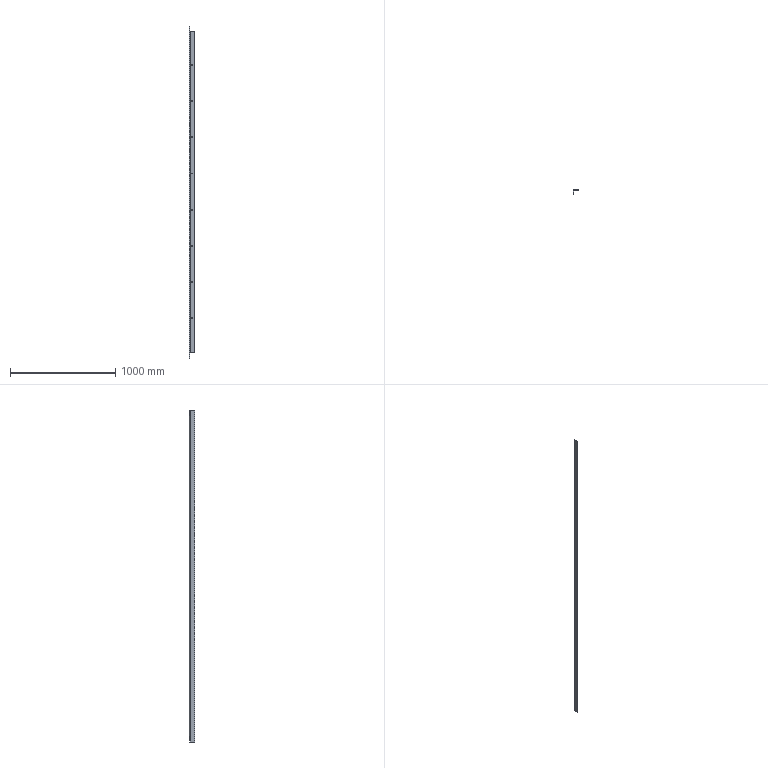Part | SolidWorks | features BaseBody 1 | 1 solid | 30 faces | box 50 x 50 x 3151 mm | volume 1714556 mm3 | cylinder 18 | plane 12 | commonest cylinder face diameters 9 x16 1.473 x1 13.473 x1
STEP:
#1=CARTESIAN_POINT('',(26.,50.,383.5));
#2=VERTEX_POINT('',#1);
#3=CARTESIAN_POINT('',(26.,50.,374.5));
#4=VERTEX_POINT('',#3);
#5=CARTESIAN_POINT('',(26.,50.,379.));
#6=DIRECTION('',(0.,-1.,0.));
#7=DIRECTION('',(0.,0.,-1.));
#8=AXIS2_PLACEMENT_3D('',#5,#6,#7);
#9=CIRCLE('',#8,4.5);
#10=EDGE_CURVE('',#2,#4,#9,.T.);
#11=ORIENTED_EDGE('',*,*,#10,.F.);
#12=CARTESIAN_POINT('',(26.,44.,383.5));
#13=VERTEX_POINT('',#12);
#14=CARTESIAN_POINT('',(26.,50.,383.5));
#15=DIRECTION('',(0.,-1.,0.));
#16=VECTOR('',#15,1000.);
#17=LINE('',#14,#16);
#18=EDGE_CURVE('',#2,#13,#17,.T.);
#19=ORIENTED_EDGE('',*,*,#18,.T.);
#20=CARTESIAN_POINT('',(26.,44.,374.5));
#21=VERTEX_POINT('',#20);
#22=CARTESIAN_POINT('',(26.,44.,379.));
#23=DIRECTION('',(0.,-1.,0.));
#24=DIRECTION('',(0.,0.,-1.));
#25=AXIS2_PLACEMENT_3D('',#22,#23,#24);
#26=CIRCLE('',#25,4.5);
#27=EDGE_CURVE('',#13,#21,#26,.T.);
#28=ORIENTED_EDGE('',*,*,#27,.T.);
#29=CARTESIAN_POINT('',(26.,50.,374.5));
#30=DIRECTION('',(0.,-1.,0.));
#31=VECTOR('',#30,1000.);
#32=LINE('',#29,#31);
#33=EDGE_CURVE('',#4,#21,#32,.T.);
#34=ORIENTED_EDGE('',*,*,#33,.F.);
#35=EDGE_LOOP('',(#11,#19,#28,#34));
#36=FACE_OUTER_BOUND('',#35,.T.);
#37=CARTESIAN_POINT('',(26.,50.,379.));
#38=DIRECTION('',(0.,-1.,0.));
#39=DIRECTION('',(0.,0.,-1.));
#40=AXIS2_PLACEMENT_3D('',#37,#38,#39);
#41=CYLINDRICAL_SURFACE('',#40,4.5);
#42=ADVANCED_FACE('',(#36),#41,.F.);
#43=CARTESIAN_POINT('',(26.,50.,726.5));
#44=VERTEX_POINT('',#43);
#45=CARTESIAN_POINT('',(26.,50.,717.5));
#46=VERTEX_POINT('',#45);
#47=CARTESIAN_POINT('',(26.,50.,722.));
#48=DIRECTION('',(0.,-1.,0.));
#49=DIRECTION('',(0.,0.,-1.));
#50=AXIS2_PLACEMENT_3D('',#47,#48,#49);
#51=CIRCLE('',#50,4.5);
#52=EDGE_CURVE('',#44,#46,#51,.T.);
#53=ORIENTED_EDGE('',*,*,#52,.F.);
#54=CARTESIAN_POINT('',(26.,44.,726.5));
#55=VERTEX_POINT('',#54);
#56=CARTESIAN_POINT('',(26.,50.,726.5));
#57=DIRECTION('',(0.,-1.,0.));
#58=VECTOR('',#57,1000.);
#59=LINE('',#56,#58);
#60=EDGE_CURVE('',#44,#55,#59,.T.);
#61=ORIENTED_EDGE('',*,*,#60,.T.);
#62=CARTESIAN_POINT('',(26.,44.,717.5));
#63=VERTEX_POINT('',#62);
#64=CARTESIAN_POINT('',(26.,44.,722.));
#65=DIRECTION('',(0.,-1.,0.));
#66=DIRECTION('',(0.,0.,-1.));
#67=AXIS2_PLACEMENT_3D('',#64,#65,#66);
#68=CIRCLE('',#67,4.5);
#69=EDGE_CURVE('',#55,#63,#68,.T.);
#70=ORIENTED_EDGE('',*,*,#69,.T.);
#71=CARTESIAN_POINT('',(26.,50.,717.5));
#72=DIRECTION('',(0.,-1.,0.));
#73=VECTOR('',#72,1000.);
#74=LINE('',#71,#73);
#75=EDGE_CURVE('',#46,#63,#74,.T.);
#76=ORIENTED_EDGE('',*,*,#75,.F.);
#77=EDGE_LOOP('',(#53,#61,#70,#76));
#78=FACE_OUTER_BOUND('',#77,.T.);
#79=CARTESIAN_POINT('',(26.,50.,722.));
#80=DIRECTION('',(0.,-1.,0.));
#81=DIRECTION('',(0.,0.,-1.));
#82=AXIS2_PLACEMENT_3D('',#79,#80,#81);
#83=CYLINDRICAL_SURFACE('',#82,4.5);
#84=ADVANCED_FACE('',(#78),#83,.F.);
#85=CARTESIAN_POINT('',(26.,50.,1069.5));
#86=VERTEX_POINT('',#85);
#87=CARTESIAN_POINT('',(26.,50.,1060.5));
#88=VERTEX_POINT('',#87);
#89=CARTESIAN_POINT('',(26.,50.,1065.));
#90=DIRECTION('',(0.,-1.,0.));
#91=DIRECTION('',(0.,0.,-1.));
#92=AXIS2_PLACEMENT_3D('',#89,#90,#91);
#93=CIRCLE('',#92,4.5);
#94=EDGE_CURVE('',#86,#88,#93,.T.);
#95=ORIENTED_EDGE('',*,*,#94,.F.);
#96=CARTESIAN_POINT('',(26.,44.,1069.5));
#97=VERTEX_POINT('',#96);
#98=CARTESIAN_POINT('',(26.,50.,1069.5));
#99=DIRECTION('',(0.,-1.,0.));
#100=VECTOR('',#99,1000.);
#101=LINE('',#98,#100);
#102=EDGE_CURVE('',#86,#97,#101,.T.);
#103=ORIENTED_EDGE('',*,*,#102,.T.);
#104=CARTESIAN_POINT('',(26.,44.,1060.5));
#105=VERTEX_POINT('',#104);
#106=CARTESIAN_POINT('',(26.,44.,1065.));
#107=DIRECTION('',(0.,-1.,0.));
#108=DIRECTION('',(0.,0.,-1.));
#109=AXIS2_PLACEMENT_3D('',#106,#107,#108);
#110=CIRCLE('',#109,4.5);
#111=EDGE_CURVE('',#97,#105,#110,.T.);
#112=ORIENTED_EDGE('',*,*,#111,.T.);
#113=CARTESIAN_POINT('',(26.,50.,1060.5));
#114=DIRECTION('',(0.,-1.,0.));
#115=VECTOR('',#114,1000.);
#116=LINE('',#113,#115);
#117=EDGE_CURVE('',#88,#105,#116,.T.);
#118=ORIENTED_EDGE('',*,*,#117,.F.);
#119=EDGE_LOOP('',(#95,#103,#112,#118));
#120=FACE_OUTER_BOUND('',#119,.T.);
#121=CARTESIAN_POINT('',(26.,50.,1065.));
#122=DIRECTION('',(0.,-1.,0.));
#123=DIRECTION('',(0.,0.,-1.));
#124=AXIS2_PLACEMENT_3D('',#121,#122,#123);
#125=CYLINDRICAL_SURFACE('',#124,4.5);
#126=ADVANCED_FACE('',(#120),#125,.F.);
#127=CARTESIAN_POINT('',(26.,50.,1412.5));
#128=VERTEX_POINT('',#127);
#129=CARTESIAN_POINT('',(26.,50.,1403.5));
#130=VERTEX_POINT('',#129);
#131=CARTESIAN_POINT('',(26.,50.,1408.));
#132=DIRECTION('',(0.,-1.,0.));
#133=DIRECTION('',(0.,0.,-1.));
#134=AXIS2_PLACEMENT_3D('',#131,#132,#133);
#135=CIRCLE('',#134,4.5);
#136=EDGE_CURVE('',#128,#130,#135,.T.);
#137=ORIENTED_EDGE('',*,*,#136,.F.);
#138=CARTESIAN_POINT('',(26.,44.,1412.5));
#139=VERTEX_POINT('',#138);
#140=CARTESIAN_POINT('',(26.,50.,1412.5));
#141=DIRECTION('',(0.,-1.,0.));
#142=VECTOR('',#141,1000.);
#143=LINE('',#140,#142);
#144=EDGE_CURVE('',#128,#139,#143,.T.);
#145=ORIENTED_EDGE('',*,*,#144,.T.);
#146=CARTESIAN_POINT('',(26.,44.,1403.5));
#147=VERTEX_POINT('',#146);
#148=CARTESIAN_POINT('',(26.,44.,1408.));
#149=DIRECTION('',(0.,-1.,0.));
#150=DIRECTION('',(0.,0.,-1.));
#151=AXIS2_PLACEMENT_3D('',#148,#149,#150);
#152=CIRCLE('',#151,4.5);
#153=EDGE_CURVE('',#139,#147,#152,.T.);
#154=ORIENTED_EDGE('',*,*,#153,.T.);
#155=CARTESIAN_POINT('',(26.,50.,1403.5));
#156=DIRECTION('',(0.,-1.,0.));
#157=VECTOR('',#156,1000.);
#158=LINE('',#155,#157);
#159=EDGE_CURVE('',#130,#147,#158,.T.);
#160=ORIENTED_EDGE('',*,*,#159,.F.);
#161=EDGE_LOOP('',(#137,#145,#154,#160));
#162=FACE_OUTER_BOUND('',#161,.T.);
#163=CARTESIAN_POINT('',(26.,50.,1408.));
#164=DIRECTION('',(0.,-1.,0.));
#165=DIRECTION('',(0.,0.,-1.));
#166=AXIS2_PLACEMENT_3D('',#163,#164,#165);
#167=CYLINDRICAL_SURFACE('',#166,4.5);
#168=ADVANCED_FACE('',(#162),#167,.F.);
#169=CARTESIAN_POINT('',(26.,50.,1755.5));
#170=VERTEX_POINT('',#169);
#171=CARTESIAN_POINT('',(26.,50.,1746.5));
#172=VERTEX_POINT('',#171);
#173=CARTESIAN_POINT('',(26.,50.,1751.));
#174=DIRECTION('',(0.,-1.,0.));
#175=DIRECTION('',(0.,0.,-1.));
#176=AXIS2_PLACEMENT_3D('',#173,#174,#175);
#177=CIRCLE('',#176,4.5);
#178=EDGE_CURVE('',#170,#172,#177,.T.);
#179=ORIENTED_EDGE('',*,*,#178,.F.);
#180=CARTESIAN_POINT('',(26.,44.,1755.5));
#181=VERTEX_POINT('',#180);
#182=CARTESIAN_POINT('',(26.,50.,1755.5));
#183=DIRECTION('',(0.,-1.,0.));
#184=VECTOR('',#183,1000.);
#185=LINE('',#182,#184);
#186=EDGE_CURVE('',#170,#181,#185,.T.);
#187=ORIENTED_EDGE('',*,*,#186,.T.);
#188=CARTESIAN_POINT('',(26.,44.,1746.5));
#189=VERTEX_POINT('',#188);
#190=CARTESIAN_POINT('',(26.,44.,1751.));
#191=DIRECTION('',(0.,-1.,0.));
#192=DIRECTION('',(0.,0.,-1.));
#193=AXIS2_PLACEMENT_3D('',#190,#191,#192);
#194=CIRCLE('',#193,4.5);
#195=EDGE_CURVE('',#181,#189,#194,.T.);
#196=ORIENTED_EDGE('',*,*,#195,.T.);
#197=CARTESIAN_POINT('',(26.,50.,1746.5));
#198=DIRECTION('',(0.,-1.,0.));
#199=VECTOR('',#198,1000.);
#200=LINE('',#197,#199);
#201=EDGE_CURVE('',#172,#189,#200,.T.);
#202=ORIENTED_EDGE('',*,*,#201,.F.);
#203=EDGE_LOOP('',(#179,#187,#196,#202));
#204=FACE_OUTER_BOUND('',#203,.T.);
#205=CARTESIAN_POINT('',(26.,50.,1751.));
#206=DIRECTION('',(0.,-1.,0.));
#207=DIRECTION('',(0.,0.,-1.));
#208=AXIS2_PLACEMENT_3D('',#205,#206,#207);
#209=CYLINDRICAL_SURFACE('',#208,4.5);
#210=ADVANCED_FACE('',(#204),#209,.F.);
#211=CARTESIAN_POINT('',(26.,50.,2098.5));
#212=VERTEX_POINT('',#211);
#213=CARTESIAN_POINT('',(26.,50.,2089.5));
#214=VERTEX_POINT('',#213);
#215=CARTESIAN_POINT('',(26.,50.,2094.));
#216=DIRECTION('',(0.,-1.,0.));
#217=DIRECTION('',(0.,0.,-1.));
#218=AXIS2_PLACEMENT_3D('',#215,#216,#217);
#219=CIRCLE('',#218,4.5);
#220=EDGE_CURVE('',#212,#214,#219,.T.);
#221=ORIENTED_EDGE('',*,*,#220,.F.);
#222=CARTESIAN_POINT('',(26.,44.,2098.5));
#223=VERTEX_POINT('',#222);
#224=CARTESIAN_POINT('',(26.,50.,2098.5));
#225=DIRECTION('',(0.,-1.,0.));
#226=VECTOR('',#225,1000.);
#227=LINE('',#224,#226);
#228=EDGE_CURVE('',#212,#223,#227,.T.);
#229=ORIENTED_EDGE('',*,*,#228,.T.);
#230=CARTESIAN_POINT('',(26.,44.,2089.5));
#231=VERTEX_POINT('',#230);
#232=CARTESIAN_POINT('',(26.,44.,2094.));
#233=DIRECTION('',(0.,-1.,0.));
#234=DIRECTION('',(0.,0.,-1.));
#235=AXIS2_PLACEMENT_3D('',#232,#233,#234);
#236=CIRCLE('',#235,4.5);
#237=EDGE_CURVE('',#223,#231,#236,.T.);
#238=ORIENTED_EDGE('',*,*,#237,.T.);
#239=CARTESIAN_POINT('',(26.,50.,2089.5));
#240=DIRECTION('',(0.,-1.,0.));
#241=VECTOR('',#240,1000.);
#242=LINE('',#239,#241);
#243=EDGE_CURVE('',#214,#231,#242,.T.);
#244=ORIENTED_EDGE('',*,*,#243,.F.);
#245=EDGE_LOOP('',(#221,#229,#238,#244));
#246=FACE_OUTER_BOUND('',#245,.T.);
#247=CARTESIAN_POINT('',(26.,50.,2094.));
#248=DIRECTION('',(0.,-1.,0.));
#249=DIRECTION('',(0.,0.,-1.));
#250=AXIS2_PLACEMENT_3D('',#247,#248,#249);
#251=CYLINDRICAL_SURFACE('',#250,4.5);
#252=ADVANCED_FACE('',(#246),#251,.F.);
#253=CARTESIAN_POINT('',(26.,50.,2441.5));
#254=VERTEX_POINT('',#253);
#255=CARTESIAN_POINT('',(26.,50.,2432.5));
#256=VERTEX_POINT('',#255);
#257=CARTESIAN_POINT('',(26.,50.,2437.));
#258=DIRECTION('',(0.,-1.,0.));
#259=DIRECTION('',(0.,0.,-1.));
#260=AXIS2_PLACEMENT_3D('',#257,#258,#259);
#261=CIRCLE('',#260,4.5);
#262=EDGE_CURVE('',#254,#256,#261,.T.);
#263=ORIENTED_EDGE('',*,*,#262,.F.);
#264=CARTESIAN_POINT('',(26.,44.,2441.5));
#265=VERTEX_POINT('',#264);
#266=CARTESIAN_POINT('',(26.,50.,2441.5));
#267=DIRECTION('',(0.,-1.,0.));
#268=VECTOR('',#267,1000.);
#269=LINE('',#266,#268);
#270=EDGE_CURVE('',#254,#265,#269,.T.);
#271=ORIENTED_EDGE('',*,*,#270,.T.);
#272=CARTESIAN_POINT('',(26.,44.,2432.5));
#273=VERTEX_POINT('',#272);
#274=CARTESIAN_POINT('',(26.,44.,2437.));
#275=DIRECTION('',(0.,-1.,0.));
#276=DIRECTION('',(0.,0.,-1.));
#277=AXIS2_PLACEMENT_3D('',#274,#275,#276);
#278=CIRCLE('',#277,4.5);
#279=EDGE_CURVE('',#265,#273,#278,.T.);
#280=ORIENTED_EDGE('',*,*,#279,.T.);
#281=CARTESIAN_POINT('',(26.,50.,2432.5));
#282=DIRECTION('',(0.,-1.,0.));
#283=VECTOR('',#282,1000.);
#284=LINE('',#281,#283);
#285=EDGE_CURVE('',#256,#273,#284,.T.);
#286=ORIENTED_EDGE('',*,*,#285,.F.);
#287=EDGE_LOOP('',(#263,#271,#280,#286));
#288=FACE_OUTER_BOUND('',#287,.T.);
#289=CARTESIAN_POINT('',(26.,50.,2437.));
#290=DIRECTION('',(0.,-1.,0.));
#291=DIRECTION('',(0.,0.,-1.));
#292=AXIS2_PLACEMENT_3D('',#289,#290,#291);
#293=CYLINDRICAL_SURFACE('',#292,4.5);
#294=ADVANCED_FACE('',(#288),#293,.F.);
#295=CARTESIAN_POINT('',(26.,50.,2784.5));
#296=VERTEX_POINT('',#295);
#297=CARTESIAN_POINT('',(26.,50.,2775.5));
#298=VERTEX_POINT('',#297);
#299=CARTESIAN_POINT('',(26.,50.,2780.));
#300=DIRECTION('',(0.,-1.,0.));
#301=DIRECTION('',(0.,0.,-1.));
#302=AXIS2_PLACEMENT_3D('',#299,#300,#301);
#303=CIRCLE('',#302,4.5);
#304=EDGE_CURVE('',#296,#298,#303,.T.);
#305=ORIENTED_EDGE('',*,*,#304,.F.);
#306=CARTESIAN_POINT('',(26.,44.,2784.5));
#307=VERTEX_POINT('',#306);
#308=CARTESIAN_POINT('',(26.,50.,2784.5));
#309=DIRECTION('',(0.,-1.,0.));
#310=VECTOR('',#309,1000.);
#311=LINE('',#308,#310);
#312=EDGE_CURVE('',#296,#307,#311,.T.);
#313=ORIENTED_EDGE('',*,*,#312,.T.);
#314=CARTESIAN_POINT('',(26.,44.,2775.5));
#315=VERTEX_POINT('',#314);
#316=CARTESIAN_POINT('',(26.,44.,2780.));
#317=DIRECTION('',(0.,-1.,0.));
#318=DIRECTION('',(0.,0.,-1.));
#319=AXIS2_PLACEMENT_3D('',#316,#317,#318);
#320=CIRCLE('',#319,4.5);
#321=EDGE_CURVE('',#307,#315,#320,.T.);
#322=ORIENTED_EDGE('',*,*,#321,.T.);
#323=CARTESIAN_POINT('',(26.,50.,2775.5));
#324=DIRECTION('',(0.,-1.,0.));
#325=VECTOR('',#324,1000.);
#326=LINE('',#323,#325);
#327=EDGE_CURVE('',#298,#315,#326,.T.);
#328=ORIENTED_EDGE('',*,*,#327,.F.);
#329=EDGE_LOOP('',(#305,#313,#322,#328));
#330=FACE_OUTER_BOUND('',#329,.T.);
#331=CARTESIAN_POINT('',(26.,50.,2780.));
#332=DIRECTION('',(0.,-1.,0.));
#333=DIRECTION('',(0.,0.,-1.));
#334=AXIS2_PLACEMENT_3D('',#331,#332,#333);
#335=CYLINDRICAL_SURFACE('',#334,4.5);
#336=ADVANCED_FACE('',(#330),#335,.F.);
#337=CARTESIAN_POINT('',(6.,43.263,3151.));
#338=VERTEX_POINT('',#337);
#339=CARTESIAN_POINT('',(6.,43.263,0.));
#340=VERTEX_POINT('',#339);
#341=CARTESIAN_POINT('',(6.,43.263,3151.));
#342=DIRECTION('',(0.,0.,-1.));
#343=VECTOR('',#342,1000.);
#344=LINE('',#341,#343);
#345=EDGE_CURVE('',#338,#340,#344,.T.);
#346=ORIENTED_EDGE('',*,*,#345,.F.);
#347=CARTESIAN_POINT('',(6.,0.,3151.));
#348=VERTEX_POINT('',#347);
#349=CARTESIAN_POINT('',(6.,0.,3151.));
#350=DIRECTION('',(0.,1.,0.));
#351=VECTOR('',#350,1000.);
#352=LINE('',#349,#351);
#353=EDGE_CURVE('',#348,#338,#352,.T.);
#354=ORIENTED_EDGE('',*,*,#353,.F.);
#355=CARTESIAN_POINT('',(6.,0.,0.));
#356=VERTEX_POINT('',#355);
#357=CARTESIAN_POINT('',(6.,0.,3151.));
#358=DIRECTION('',(0.,0.,1.));
#359=VECTOR('',#358,1000.);
#360=LINE('',#357,#359);
#361=EDGE_CURVE('',#356,#348,#360,.T.);
#362=ORIENTED_EDGE('',*,*,#361,.F.);
#363=CARTESIAN_POINT('',(6.,0.,0.));
#364=DIRECTION('',(0.,-1.,0.));
#365=VECTOR('',#364,1000.);
#366=LINE('',#363,#365);
#367=EDGE_CURVE('',#340,#356,#366,.T.);
#368=ORIENTED_EDGE('',*,*,#367,.F.);
#369=EDGE_LOOP('',(#346,#354,#362,#368));
#370=FACE_OUTER_BOUND('',#369,.T.);
#371=CARTESIAN_POINT('',(6.,0.,3151.));
#372=DIRECTION('',(-1.,0.,0.));
#373=DIRECTION('',(0.,0.,1.));
#374=AXIS2_PLACEMENT_3D('',#371,#372,#373);
#375=PLANE('',#374);
#376=ADVANCED_FACE('',(#370),#375,.F.);
#377=ORIENTED_EDGE('',*,*,#367,.T.);
#378=CARTESIAN_POINT('',(0.,0.,0.));
#379=VERTEX_POINT('',#378);
#380=CARTESIAN_POINT('',(6.737,0.,0.));
#381=DIRECTION('',(-1.,0.,0.));
#382=VECTOR('',#381,1000.);
#383=LINE('',#380,#382);
#384=EDGE_CURVE('',#356,#379,#383,.T.);
#385=ORIENTED_EDGE('',*,*,#384,.T.);
#386=CARTESIAN_POINT('',(0.,43.263,0.));
#387=VERTEX_POINT('',#386);
#388=CARTESIAN_POINT('',(0.,44.,0.));
#389=DIRECTION('',(0.,1.,0.));
#390=VECTOR('',#389,1000.);
#391=LINE('',#388,#390);
#392=EDGE_CURVE('',#379,#387,#391,.T.);
#393=ORIENTED_EDGE('',*,*,#392,.T.);
#394=CARTESIAN_POINT('',(0.04039,44.,0.));
#395=VERTEX_POINT('',#394);
#396=CARTESIAN_POINT('',(6.737,43.263,0.));
#397=DIRECTION('',(0.,0.,1.));
#398=DIRECTION('',(-1.,0.,0.));
#399=AXIS2_PLACEMENT_3D('',#396,#397,#398);
#400=CIRCLE('',#399,6.737);
#401=EDGE_CURVE('',#395,#387,#400,.T.);
#402=ORIENTED_EDGE('',*,*,#401,.F.);
#403=CARTESIAN_POINT('',(6.004,43.344,0.));
#404=VERTEX_POINT('',#403);
#405=CARTESIAN_POINT('',(0.04039,44.,0.));
#406=DIRECTION('',(0.994,-0.1093,0.));
#407=VECTOR('',#406,1000.);
#408=LINE('',#405,#407);
#409=EDGE_CURVE('',#395,#404,#408,.T.);
#410=ORIENTED_EDGE('',*,*,#409,.T.);
#411=CARTESIAN_POINT('',(6.737,43.263,0.));
#412=DIRECTION('',(0.,0.,1.));
#413=DIRECTION('',(-1.,0.,0.));
#414=AXIS2_PLACEMENT_3D('',#411,#412,#413);
#415=CIRCLE('',#414,0.7366);
#416=EDGE_CURVE('',#404,#340,#415,.T.);
#417=ORIENTED_EDGE('',*,*,#416,.T.);
#418=EDGE_LOOP('',(#377,#385,#393,#402,#410,#417));
#419=FACE_OUTER_BOUND('',#418,.T.);
#420=CARTESIAN_POINT('',(6.737,44.,0.));
#421=DIRECTION('',(0.,0.,-1.));
#422=DIRECTION('',(-1.,0.,0.));
#423=AXIS2_PLACEMENT_3D('',#420,#421,#422);
#424=PLANE('',#423);
#425=ADVANCED_FACE('',(#419),#424,.T.);
#426=CARTESIAN_POINT('',(6.004,43.344,3151.));
#427=VERTEX_POINT('',#426);
#428=CARTESIAN_POINT('',(6.737,43.263,3151.));
#429=DIRECTION('',(0.,0.,-1.));
#430=DIRECTION('',(-1.,0.,0.));
#431=AXIS2_PLACEMENT_3D('',#428,#429,#430);
#432=CIRCLE('',#431,0.7366);
#433=EDGE_CURVE('',#338,#427,#432,.T.);
#434=ORIENTED_EDGE('',*,*,#433,.F.);
#435=ORIENTED_EDGE('',*,*,#345,.T.);
#436=ORIENTED_EDGE('',*,*,#416,.F.);
#437=CARTESIAN_POINT('',(6.004,43.344,50.));
#438=VERTEX_POINT('',#437);
#439=CARTESIAN_POINT('',(6.004,43.344,3151.));
#440=DIRECTION('',(0.,0.,-1.));
#441=VECTOR('',#440,1000.);
#442=LINE('',#439,#441);
#443=EDGE_CURVE('',#438,#404,#442,.T.);
#444=ORIENTED_EDGE('',*,*,#443,.F.);
#445=CARTESIAN_POINT('',(6.737,44.,50.));
#446=VERTEX_POINT('',#445);
#447=CARTESIAN_POINT('',(6.737,43.263,50.));
#448=DIRECTION('',(0.,0.,1.));
#449=DIRECTION('',(-1.,0.,0.));
#450=AXIS2_PLACEMENT_3D('',#447,#448,#449);
#451=CIRCLE('',#450,0.7366);
#452=EDGE_CURVE('',#446,#438,#451,.T.);
#453=ORIENTED_EDGE('',*,*,#452,.F.);
#454=CARTESIAN_POINT('',(6.737,44.,3101.));
#455=VERTEX_POINT('',#454);
#456=CARTESIAN_POINT('',(6.737,44.,3151.));
#457=DIRECTION('',(0.,0.,-1.));
#458=VECTOR('',#457,1000.);
#459=LINE('',#456,#458);
#460=EDGE_CURVE('',#455,#446,#459,.T.);
#461=ORIENTED_EDGE('',*,*,#460,.F.);
#462=CARTESIAN_POINT('',(6.004,43.344,3101.));
#463=VERTEX_POINT('',#462);
#464=CARTESIAN_POINT('',(6.737,43.263,3101.));
#465=DIRECTION('',(0.,0.,-1.));
#466=DIRECTION('',(-1.,0.,0.));
#467=AXIS2_PLACEMENT_3D('',#464,#465,#466);
#468=CIRCLE('',#467,0.7366);
#469=EDGE_CURVE('',#463,#455,#468,.T.);
#470=ORIENTED_EDGE('',*,*,#469,.F.);
#471=CARTESIAN_POINT('',(6.004,43.344,3151.));
#472=DIRECTION('',(0.,0.,-1.));
#473=VECTOR('',#472,1000.);
#474=LINE('',#471,#473);
#475=EDGE_CURVE('',#427,#463,#474,.T.);
#476=ORIENTED_EDGE('',*,*,#475,.F.);
#477=EDGE_LOOP('',(#434,#435,#436,#444,#453,#461,#470,#476));
#478=FACE_OUTER_BOUND('',#477,.T.);
#479=CARTESIAN_POINT('',(6.737,43.263,3151.));
#480=DIRECTION('',(0.,0.,-1.));
#481=DIRECTION('',(-1.,0.,0.));
#482=AXIS2_PLACEMENT_3D('',#479,#480,#481);
#483=CYLINDRICAL_SURFACE('',#482,0.7366);
#484=ADVANCED_FACE('',(#478),#483,.F.);
#485=CARTESIAN_POINT('',(0.,43.263,3151.));
#486=VERTEX_POINT('',#485);
#487=CARTESIAN_POINT('',(0.,0.,3151.));
#488=VERTEX_POINT('',#487);
#489=CARTESIAN_POINT('',(0.,43.263,3151.));
#490=DIRECTION('',(0.,-1.,0.));
#491=VECTOR('',#490,1000.);
#492=LINE('',#489,#491);
#493=EDGE_CURVE('',#486,#488,#492,.T.);
#494=ORIENTED_EDGE('',*,*,#493,.T.);
#495=CARTESIAN_POINT('',(6.737,0.,3151.));
#496=DIRECTION('',(1.,0.,0.));
#497=VECTOR('',#496,1000.);
#498=LINE('',#495,#497);
#499=EDGE_CURVE('',#488,#348,#498,.T.);
#500=ORIENTED_EDGE('',*,*,#499,.T.);
#501=ORIENTED_EDGE('',*,*,#353,.T.);
#502=ORIENTED_EDGE('',*,*,#433,.T.);
#503=CARTESIAN_POINT('',(0.04039,44.,3151.));
#504=VERTEX_POINT('',#503);
#505=CARTESIAN_POINT('',(0.04039,44.,3151.));
#506=DIRECTION('',(0.994,-0.1093,0.));
#507=VECTOR('',#506,1000.);
#508=LINE('',#505,#507);
#509=EDGE_CURVE('',#504,#427,#508,.T.);
#510=ORIENTED_EDGE('',*,*,#509,.F.);
#511=CARTESIAN_POINT('',(6.737,43.263,3151.));
#512=DIRECTION('',(0.,0.,1.));
#513=DIRECTION('',(-1.,0.,0.));
#514=AXIS2_PLACEMENT_3D('',#511,#512,#513);
#515=CIRCLE('',#514,6.737);
#516=EDGE_CURVE('',#504,#486,#515,.T.);
#517=ORIENTED_EDGE('',*,*,#516,.T.);
#518=EDGE_LOOP('',(#494,#500,#501,#502,#510,#517));
#519=FACE_OUTER_BOUND('',#518,.T.);
#520=CARTESIAN_POINT('',(6.737,43.263,3151.));
#521=DIRECTION('',(0.,0.,1.));
#522=DIRECTION('',(1.,0.,0.));
#523=AXIS2_PLACEMENT_3D('',#520,#521,#522);
#524=PLANE('',#523);
#525=ADVANCED_FACE('',(#519),#524,.T.);
#526=ORIENTED_EDGE('',*,*,#499,.F.);
#527=CARTESIAN_POINT('',(0.,0.,3151.));
#528=DIRECTION('',(0.,0.,-1.));
#529=VECTOR('',#528,1000.);
#530=LINE('',#527,#529);
#531=EDGE_CURVE('',#488,#379,#530,.T.);
#532=ORIENTED_EDGE('',*,*,#531,.T.);
#533=ORIENTED_EDGE('',*,*,#384,.F.);
#534=ORIENTED_EDGE('',*,*,#361,.T.);
#535=EDGE_LOOP('',(#526,#532,#533,#534));
#536=FACE_OUTER_BOUND('',#535,.T.);
#537=CARTESIAN_POINT('',(6.,0.,3151.));
#538=DIRECTION('',(0.,-1.,0.));
#539=DIRECTION('',(0.,0.,-1.));
#540=AXIS2_PLACEMENT_3D('',#537,#538,#539);
#541=PLANE('',#540);
#542=ADVANCED_FACE('',(#536),#541,.T.);
#543=ORIENTED_EDGE('',*,*,#493,.F.);
#544=CARTESIAN_POINT('',(0.,43.263,3151.));
#545=DIRECTION('',(0.,0.,-1.));
#546=VECTOR('',#545,1000.);
#547=LINE('',#544,#546);
#548=EDGE_CURVE('',#486,#387,#547,.T.);
#549=ORIENTED_EDGE('',*,*,#548,.T.);
#550=ORIENTED_EDGE('',*,*,#392,.F.);
#551=ORIENTED_EDGE('',*,*,#531,.F.);
#552=EDGE_LOOP('',(#543,#549,#550,#551));
#553=FACE_OUTER_BOUND('',#552,.T.);
#554=CARTESIAN_POINT('',(0.,0.,3151.));
#555=DIRECTION('',(-1.,0.,0.));
#556=DIRECTION('',(0.,0.,1.));
#557=AXIS2_PLACEMENT_3D('',#554,#555,#556);
#558=PLANE('',#557);
#559=ADVANCED_FACE('',(#553),#558,.T.);
#560=ORIENTED_EDGE('',*,*,#509,.T.);
#561=ORIENTED_EDGE('',*,*,#475,.T.);
#562=CARTESIAN_POINT('',(0.04039,44.,3101.));
#563=VERTEX_POINT('',#562);
#564=CARTESIAN_POINT('',(0.04039,44.,3101.));
#565=DIRECTION('',(-0.994,0.1093,0.));
#566=VECTOR('',#565,1000.);
#567=LINE('',#564,#566);
#568=EDGE_CURVE('',#463,#563,#567,.T.);
#569=ORIENTED_EDGE('',*,*,#568,.T.);
#570=CARTESIAN_POINT('',(0.04039,44.,3126.));
#571=DIRECTION('',(0.,0.,1.));
#572=VECTOR('',#571,1000.);
#573=LINE('',#570,#572);
#574=EDGE_CURVE('',#563,#504,#573,.T.);
#575=ORIENTED_EDGE('',*,*,#574,.T.);
#576=EDGE_LOOP('',(#560,#561,#569,#575));
#577=FACE_OUTER_BOUND('',#576,.T.);
#578=CARTESIAN_POINT('',(0.04039,44.,3126.));
#579=DIRECTION('',(0.1093,0.994,0.));
#580=DIRECTION('',(-0.994,0.1093,0.));
#581=AXIS2_PLACEMENT_3D('',#578,#579,#580);
#582=PLANE('',#581);
#583=ADVANCED_FACE('',(#577),#582,.T.);
#584=ORIENTED_EDGE('',*,*,#409,.F.);
#585=CARTESIAN_POINT('',(0.04039,44.,50.));
#586=VERTEX_POINT('',#585);
#587=CARTESIAN_POINT('',(0.04039,44.,25.));
#588=DIRECTION('',(0.,0.,1.));
#589=VECTOR('',#588,1000.);
#590=LINE('',#587,#589);
#591=EDGE_CURVE('',#395,#586,#590,.T.);
#592=ORIENTED_EDGE('',*,*,#591,.T.);
#593=CARTESIAN_POINT('',(0.04039,44.,50.));
#594=DIRECTION('',(0.994,-0.1093,0.));
#595=VECTOR('',#594,1000.);
#596=LINE('',#593,#595);
#597=EDGE_CURVE('',#586,#438,#596,.T.);
#598=ORIENTED_EDGE('',*,*,#597,.T.);
#599=ORIENTED_EDGE('',*,*,#443,.T.);
#600=EDGE_LOOP('',(#584,#592,#598,#599));
#601=FACE_OUTER_BOUND('',#600,.T.);
#602=CARTESIAN_POINT('',(0.04039,44.,25.));
#603=DIRECTION('',(0.1093,0.994,0.));
#604=DIRECTION('',(-0.994,0.1093,0.));
#605=AXIS2_PLACEMENT_3D('',#602,#603,#604);
#606=PLANE('',#605);
#607=ADVANCED_FACE('',(#601),#606,.T.);
#608=ORIENTED_EDGE('',*,*,#460,.T.);
#609=CARTESIAN_POINT('',(50.,44.,50.));
#610=VERTEX_POINT('',#609);
#611=CARTESIAN_POINT('',(0.,44.,50.));
#612=DIRECTION('',(-1.,0.,0.));
#613=VECTOR('',#612,1000.);
#614=LINE('',#611,#613);
#615=EDGE_CURVE('',#610,#446,#614,.T.);
#616=ORIENTED_EDGE('',*,*,#615,.F.);
#617=CARTESIAN_POINT('',(50.,44.,3101.));
#618=VERTEX_POINT('',#617);
#619=CARTESIAN_POINT('',(50.,44.,3151.));
#620=DIRECTION('',(0.,0.,-1.));
#621=VECTOR('',#620,1000.);
#622=LINE('',#619,#621);
#623=EDGE_CURVE('',#618,#610,#622,.T.);
#624=ORIENTED_EDGE('',*,*,#623,.F.);
#625=CARTESIAN_POINT('',(0.,44.,3101.));
#626=DIRECTION('',(1.,0.,0.));
#627=VECTOR('',#626,1000.);
#628=LINE('',#625,#627);
#629=EDGE_CURVE('',#455,#618,#628,.T.);
#630=ORIENTED_EDGE('',*,*,#629,.F.);
#631=EDGE_LOOP('',(#608,#616,#624,#630));
#632=FACE_OUTER_BOUND('',#631,.T.);
#633=CARTESIAN_POINT('',(26.,44.,379.));
#634=DIRECTION('',(0.,-1.,0.));
#635=DIRECTION('',(0.,0.,-1.));
#636=AXIS2_PLACEMENT_3D('',#633,#634,#635);
#637=CIRCLE('',#636,4.5);
#638=EDGE_CURVE('',#21,#13,#637,.T.);
#639=ORIENTED_EDGE('',*,*,#638,.F.);
#640=ORIENTED_EDGE('',*,*,#27,.F.);
#641=EDGE_LOOP('',(#639,#640));
#642=FACE_BOUND('',#641,.T.);
#643=CARTESIAN_POINT('',(26.,44.,722.));
#644=DIRECTION('',(0.,-1.,0.));
#645=DIRECTION('',(0.,0.,-1.));
#646=AXIS2_PLACEMENT_3D('',#643,#644,#645);
#647=CIRCLE('',#646,4.5);
#648=EDGE_CURVE('',#63,#55,#647,.T.);
#649=ORIENTED_EDGE('',*,*,#648,.F.);
#650=ORIENTED_EDGE('',*,*,#69,.F.);
#651=EDGE_LOOP('',(#649,#650));
#652=FACE_BOUND('',#651,.T.);
#653=CARTESIAN_POINT('',(26.,44.,1065.));
#654=DIRECTION('',(0.,-1.,0.));
#655=DIRECTION('',(0.,0.,-1.));
#656=AXIS2_PLACEMENT_3D('',#653,#654,#655);
#657=CIRCLE('',#656,4.5);
#658=EDGE_CURVE('',#105,#97,#657,.T.);
#659=ORIENTED_EDGE('',*,*,#658,.F.);
#660=ORIENTED_EDGE('',*,*,#111,.F.);
#661=EDGE_LOOP('',(#659,#660));
#662=FACE_BOUND('',#661,.T.);
#663=CARTESIAN_POINT('',(26.,44.,1408.));
#664=DIRECTION('',(0.,-1.,0.));
#665=DIRECTION('',(0.,0.,-1.));
#666=AXIS2_PLACEMENT_3D('',#663,#664,#665);
#667=CIRCLE('',#666,4.5);
#668=EDGE_CURVE('',#147,#139,#667,.T.);
#669=ORIENTED_EDGE('',*,*,#668,.F.);
#670=ORIENTED_EDGE('',*,*,#153,.F.);
#671=EDGE_LOOP('',(#669,#670));
#672=FACE_BOUND('',#671,.T.);
#673=CARTESIAN_POINT('',(26.,44.,1751.));
#674=DIRECTION('',(0.,-1.,0.));
#675=DIRECTION('',(0.,0.,-1.));
#676=AXIS2_PLACEMENT_3D('',#673,#674,#675);
#677=CIRCLE('',#676,4.5);
#678=EDGE_CURVE('',#189,#181,#677,.T.);
#679=ORIENTED_EDGE('',*,*,#678,.F.);
#680=ORIENTED_EDGE('',*,*,#195,.F.);
#681=EDGE_LOOP('',(#679,#680));
#682=FACE_BOUND('',#681,.T.);
#683=CARTESIAN_POINT('',(26.,44.,2094.));
#684=DIRECTION('',(0.,-1.,0.));
#685=DIRECTION('',(0.,0.,-1.));
#686=AXIS2_PLACEMENT_3D('',#683,#684,#685);
#687=CIRCLE('',#686,4.5);
#688=EDGE_CURVE('',#231,#223,#687,.T.);
#689=ORIENTED_EDGE('',*,*,#688,.F.);
#690=ORIENTED_EDGE('',*,*,#237,.F.);
#691=EDGE_LOOP('',(#689,#690));
#692=FACE_BOUND('',#691,.T.);
#693=CARTESIAN_POINT('',(26.,44.,2437.));
#694=DIRECTION('',(0.,-1.,0.));
#695=DIRECTION('',(0.,0.,-1.));
#696=AXIS2_PLACEMENT_3D('',#693,#694,#695);
#697=CIRCLE('',#696,4.5);
#698=EDGE_CURVE('',#273,#265,#697,.T.);
#699=ORIENTED_EDGE('',*,*,#698,.F.);
#700=ORIENTED_EDGE('',*,*,#279,.F.);
#701=EDGE_LOOP('',(#699,#700));
#702=FACE_BOUND('',#701,.T.);
#703=CARTESIAN_POINT('',(26.,44.,2780.));
#704=DIRECTION('',(0.,-1.,0.));
#705=DIRECTION('',(0.,0.,-1.));
#706=AXIS2_PLACEMENT_3D('',#703,#704,#705);
#707=CIRCLE('',#706,4.5);
#708=EDGE_CURVE('',#315,#307,#707,.T.);
#709=ORIENTED_EDGE('',*,*,#708,.F.);
#710=ORIENTED_EDGE('',*,*,#321,.F.);
#711=EDGE_LOOP('',(#709,#710));
#712=FACE_BOUND('',#711,.T.);
#713=CARTESIAN_POINT('',(0.,44.,3151.));
#714=DIRECTION('',(0.,1.,0.));
#715=DIRECTION('',(0.,0.,1.));
#716=AXIS2_PLACEMENT_3D('',#713,#714,#715);
#717=PLANE('',#716);
#718=ADVANCED_FACE('',(#632,#642,#652,#662,#672,#682,#692,#702,#712),#717,.F.);
#719=ORIENTED_EDGE('',*,*,#401,.T.);
#720=ORIENTED_EDGE('',*,*,#548,.F.);
#721=ORIENTED_EDGE('',*,*,#516,.F.);
#722=ORIENTED_EDGE('',*,*,#574,.F.);
#723=CARTESIAN_POINT('',(6.737,50.,3101.));
#724=VERTEX_POINT('',#723);
#725=CARTESIAN_POINT('',(6.737,43.263,3101.));
#726=DIRECTION('',(0.,0.,-1.));
#727=DIRECTION('',(-1.,0.,0.));
#728=AXIS2_PLACEMENT_3D('',#725,#726,#727);
#729=CIRCLE('',#728,6.737);
#730=EDGE_CURVE('',#563,#724,#729,.T.);
#731=ORIENTED_EDGE('',*,*,#730,.T.);
#732=CARTESIAN_POINT('',(6.737,50.,50.));
#733=VERTEX_POINT('',#732);
#734=CARTESIAN_POINT('',(6.737,50.,3151.));
#735=DIRECTION('',(0.,0.,-1.));
#736=VECTOR('',#735,1000.);
#737=LINE('',#734,#736);
#738=EDGE_CURVE('',#724,#733,#737,.T.);
#739=ORIENTED_EDGE('',*,*,#738,.T.);
#740=CARTESIAN_POINT('',(6.737,43.263,50.));
#741=DIRECTION('',(0.,0.,1.));
#742=DIRECTION('',(-1.,0.,0.));
#743=AXIS2_PLACEMENT_3D('',#740,#741,#742);
#744=CIRCLE('',#743,6.737);
#745=EDGE_CURVE('',#733,#586,#744,.T.);
#746=ORIENTED_EDGE('',*,*,#745,.T.);
#747=ORIENTED_EDGE('',*,*,#591,.F.);
#748=EDGE_LOOP('',(#719,#720,#721,#722,#731,#739,#746,#747));
#749=FACE_OUTER_BOUND('',#748,.T.);
#750=CARTESIAN_POINT('',(6.737,43.263,3151.));
#751=DIRECTION('',(0.,0.,-1.));
#752=DIRECTION('',(-1.,0.,0.));
#753=AXIS2_PLACEMENT_3D('',#750,#751,#752);
#754=CYLINDRICAL_SURFACE('',#753,6.737);
#755=ADVANCED_FACE('',(#749),#754,.T.);
#756=ORIENTED_EDGE('',*,*,#469,.T.);
#757=ORIENTED_EDGE('',*,*,#629,.T.);
#758=CARTESIAN_POINT('',(50.,50.,3101.));
#759=VERTEX_POINT('',#758);
#760=CARTESIAN_POINT('',(50.,44.,3101.));
#761=DIRECTION('',(0.,-1.,0.));
#762=VECTOR('',#761,1000.);
#763=LINE('',#760,#762);
#764=EDGE_CURVE('',#759,#618,#763,.T.);
#765=ORIENTED_EDGE('',*,*,#764,.F.);
#766=CARTESIAN_POINT('',(50.,50.,3101.));
#767=DIRECTION('',(1.,0.,0.));
#768=VECTOR('',#767,1000.);
#769=LINE('',#766,#768);
#770=EDGE_CURVE('',#724,#759,#769,.T.);
#771=ORIENTED_EDGE('',*,*,#770,.F.);
#772=ORIENTED_EDGE('',*,*,#730,.F.);
#773=ORIENTED_EDGE('',*,*,#568,.F.);
#774=EDGE_LOOP('',(#756,#757,#765,#771,#772,#773));
#775=FACE_OUTER_BOUND('',#774,.T.);
#776=CARTESIAN_POINT('',(6.737,43.263,3101.));
#777=DIRECTION('',(0.,0.,1.));
#778=DIRECTION('',(1.,0.,0.));
#779=AXIS2_PLACEMENT_3D('',#776,#777,#778);
#780=PLANE('',#779);
#781=ADVANCED_FACE('',(#775),#780,.T.);
#782=ORIENTED_EDGE('',*,*,#597,.F.);
#783=ORIENTED_EDGE('',*,*,#745,.F.);
#784=CARTESIAN_POINT('',(50.,50.,50.));
#785=VERTEX_POINT('',#784);
#786=CARTESIAN_POINT('',(50.,50.,50.));
#787=DIRECTION('',(-1.,0.,0.));
#788=VECTOR('',#787,1000.);
#789=LINE('',#786,#788);
#790=EDGE_CURVE('',#785,#733,#789,.T.);
#791=ORIENTED_EDGE('',*,*,#790,.F.);
#792=CARTESIAN_POINT('',(50.,44.,50.));
#793=DIRECTION('',(0.,1.,0.));
#794=VECTOR('',#793,1000.);
#795=LINE('',#792,#794);
#796=EDGE_CURVE('',#610,#785,#795,.T.);
#797=ORIENTED_EDGE('',*,*,#796,.F.);
#798=ORIENTED_EDGE('',*,*,#615,.T.);
#799=ORIENTED_EDGE('',*,*,#452,.T.);
#800=EDGE_LOOP('',(#782,#783,#791,#797,#798,#799));
#801=FACE_OUTER_BOUND('',#800,.T.);
#802=CARTESIAN_POINT('',(6.737,43.263,50.));
#803=DIRECTION('',(0.,0.,-1.));
#804=DIRECTION('',(-1.,0.,0.));
#805=AXIS2_PLACEMENT_3D('',#802,#803,#804);
#806=PLANE('',#805);
#807=ADVANCED_FACE('',(#801),#806,.T.);
#808=ORIENTED_EDGE('',*,*,#623,.T.);
#809=ORIENTED_EDGE('',*,*,#796,.T.);
#810=CARTESIAN_POINT('',(50.,50.,3151.));
#811=DIRECTION('',(0.,0.,1.));
#812=VECTOR('',#811,1000.);
#813=LINE('',#810,#812);
#814=EDGE_CURVE('',#785,#759,#813,.T.);
#815=ORIENTED_EDGE('',*,*,#814,.T.);
#816=ORIENTED_EDGE('',*,*,#764,.T.);
#817=EDGE_LOOP('',(#808,#809,#815,#816));
#818=FACE_OUTER_BOUND('',#817,.T.);
#819=CARTESIAN_POINT('',(50.,50.,3151.));
#820=DIRECTION('',(1.,0.,0.));
#821=DIRECTION('',(0.,0.,-1.));
#822=AXIS2_PLACEMENT_3D('',#819,#820,#821);
#823=PLANE('',#822);
#824=ADVANCED_FACE('',(#818),#823,.T.);
#825=ORIENTED_EDGE('',*,*,#18,.F.);
#826=CARTESIAN_POINT('',(26.,50.,379.));
#827=DIRECTION('',(0.,-1.,0.));
#828=DIRECTION('',(0.,0.,-1.));
#829=AXIS2_PLACEMENT_3D('',#826,#827,#828);
#830=CIRCLE('',#829,4.5);
#831=EDGE_CURVE('',#4,#2,#830,.T.);
#832=ORIENTED_EDGE('',*,*,#831,.F.);
#833=ORIENTED_EDGE('',*,*,#33,.T.);
#834=ORIENTED_EDGE('',*,*,#638,.T.);
#835=EDGE_LOOP('',(#825,#832,#833,#834));
#836=FACE_OUTER_BOUND('',#835,.T.);
#837=CARTESIAN_POINT('',(26.,50.,379.));
#838=DIRECTION('',(0.,-1.,0.));
#839=DIRECTION('',(0.,0.,-1.));
#840=AXIS2_PLACEMENT_3D('',#837,#838,#839);
#841=CYLINDRICAL_SURFACE('',#840,4.5);
#842=ADVANCED_FACE('',(#836),#841,.F.);
#843=ORIENTED_EDGE('',*,*,#60,.F.);
#844=CARTESIAN_POINT('',(26.,50.,722.));
#845=DIRECTION('',(0.,-1.,0.));
#846=DIRECTION('',(0.,0.,-1.));
#847=AXIS2_PLACEMENT_3D('',#844,#845,#846);
#848=CIRCLE('',#847,4.5);
#849=EDGE_CURVE('',#46,#44,#848,.T.);
#850=ORIENTED_EDGE('',*,*,#849,.F.);
#851=ORIENTED_EDGE('',*,*,#75,.T.);
#852=ORIENTED_EDGE('',*,*,#648,.T.);
#853=EDGE_LOOP('',(#843,#850,#851,#852));
#854=FACE_OUTER_BOUND('',#853,.T.);
#855=CARTESIAN_POINT('',(26.,50.,722.));
#856=DIRECTION('',(0.,-1.,0.));
#857=DIRECTION('',(0.,0.,-1.));
#858=AXIS2_PLACEMENT_3D('',#855,#856,#857);
#859=CYLINDRICAL_SURFACE('',#858,4.5);
#860=ADVANCED_FACE('',(#854),#859,.F.);
#861=ORIENTED_EDGE('',*,*,#102,.F.);
#862=CARTESIAN_POINT('',(26.,50.,1065.));
#863=DIRECTION('',(0.,-1.,0.));
#864=DIRECTION('',(0.,0.,-1.));
#865=AXIS2_PLACEMENT_3D('',#862,#863,#864);
#866=CIRCLE('',#865,4.5);
#867=EDGE_CURVE('',#88,#86,#866,.T.);
#868=ORIENTED_EDGE('',*,*,#867,.F.);
#869=ORIENTED_EDGE('',*,*,#117,.T.);
#870=ORIENTED_EDGE('',*,*,#658,.T.);
#871=EDGE_LOOP('',(#861,#868,#869,#870));
#872=FACE_OUTER_BOUND('',#871,.T.);
#873=CARTESIAN_POINT('',(26.,50.,1065.));
#874=DIRECTION('',(0.,-1.,0.));
#875=DIRECTION('',(0.,0.,-1.));
#876=AXIS2_PLACEMENT_3D('',#873,#874,#875);
#877=CYLINDRICAL_SURFACE('',#876,4.5);
#878=ADVANCED_FACE('',(#872),#877,.F.);
#879=ORIENTED_EDGE('',*,*,#144,.F.);
#880=CARTESIAN_POINT('',(26.,50.,1408.));
#881=DIRECTION('',(0.,-1.,0.));
#882=DIRECTION('',(0.,0.,-1.));
#883=AXIS2_PLACEMENT_3D('',#880,#881,#882);
#884=CIRCLE('',#883,4.5);
#885=EDGE_CURVE('',#130,#128,#884,.T.);
#886=ORIENTED_EDGE('',*,*,#885,.F.);
#887=ORIENTED_EDGE('',*,*,#159,.T.);
#888=ORIENTED_EDGE('',*,*,#668,.T.);
#889=EDGE_LOOP('',(#879,#886,#887,#888));
#890=FACE_OUTER_BOUND('',#889,.T.);
#891=CARTESIAN_POINT('',(26.,50.,1408.));
#892=DIRECTION('',(0.,-1.,0.));
#893=DIRECTION('',(0.,0.,-1.));
#894=AXIS2_PLACEMENT_3D('',#891,#892,#893);
#895=CYLINDRICAL_SURFACE('',#894,4.5);
#896=ADVANCED_FACE('',(#890),#895,.F.);
#897=ORIENTED_EDGE('',*,*,#186,.F.);
#898=CARTESIAN_POINT('',(26.,50.,1751.));
#899=DIRECTION('',(0.,-1.,0.));
#900=DIRECTION('',(0.,0.,-1.));
#901=AXIS2_PLACEMENT_3D('',#898,#899,#900);
#902=CIRCLE('',#901,4.5);
#903=EDGE_CURVE('',#172,#170,#902,.T.);
#904=ORIENTED_EDGE('',*,*,#903,.F.);
#905=ORIENTED_EDGE('',*,*,#201,.T.);
#906=ORIENTED_EDGE('',*,*,#678,.T.);
#907=EDGE_LOOP('',(#897,#904,#905,#906));
#908=FACE_OUTER_BOUND('',#907,.T.);
#909=CARTESIAN_POINT('',(26.,50.,1751.));
#910=DIRECTION('',(0.,-1.,0.));
#911=DIRECTION('',(0.,0.,-1.));
#912=AXIS2_PLACEMENT_3D('',#909,#910,#911);
#913=CYLINDRICAL_SURFACE('',#912,4.5);
#914=ADVANCED_FACE('',(#908),#913,.F.);
#915=ORIENTED_EDGE('',*,*,#228,.F.);
#916=CARTESIAN_POINT('',(26.,50.,2094.));
#917=DIRECTION('',(0.,-1.,0.));
#918=DIRECTION('',(0.,0.,-1.));
#919=AXIS2_PLACEMENT_3D('',#916,#917,#918);
#920=CIRCLE('',#919,4.5);
#921=EDGE_CURVE('',#214,#212,#920,.T.);
#922=ORIENTED_EDGE('',*,*,#921,.F.);
#923=ORIENTED_EDGE('',*,*,#243,.T.);
#924=ORIENTED_EDGE('',*,*,#688,.T.);
#925=EDGE_LOOP('',(#915,#922,#923,#924));
#926=FACE_OUTER_BOUND('',#925,.T.);
#927=CARTESIAN_POINT('',(26.,50.,2094.));
#928=DIRECTION('',(0.,-1.,0.));
#929=DIRECTION('',(0.,0.,-1.));
#930=AXIS2_PLACEMENT_3D('',#927,#928,#929);
#931=CYLINDRICAL_SURFACE('',#930,4.5);
#932=ADVANCED_FACE('',(#926),#931,.F.);
#933=ORIENTED_EDGE('',*,*,#270,.F.);
#934=CARTESIAN_POINT('',(26.,50.,2437.));
#935=DIRECTION('',(0.,-1.,0.));
#936=DIRECTION('',(0.,0.,-1.));
#937=AXIS2_PLACEMENT_3D('',#934,#935,#936);
#938=CIRCLE('',#937,4.5);
#939=EDGE_CURVE('',#256,#254,#938,.T.);
#940=ORIENTED_EDGE('',*,*,#939,.F.);
#941=ORIENTED_EDGE('',*,*,#285,.T.);
#942=ORIENTED_EDGE('',*,*,#698,.T.);
#943=EDGE_LOOP('',(#933,#940,#941,#942));
#944=FACE_OUTER_BOUND('',#943,.T.);
#945=CARTESIAN_POINT('',(26.,50.,2437.));
#946=DIRECTION('',(0.,-1.,0.));
#947=DIRECTION('',(0.,0.,-1.));
#948=AXIS2_PLACEMENT_3D('',#945,#946,#947);
#949=CYLINDRICAL_SURFACE('',#948,4.5);
#950=ADVANCED_FACE('',(#944),#949,.F.);
#951=ORIENTED_EDGE('',*,*,#312,.F.);
#952=CARTESIAN_POINT('',(26.,50.,2780.));
#953=DIRECTION('',(0.,-1.,0.));
#954=DIRECTION('',(0.,0.,-1.));
#955=AXIS2_PLACEMENT_3D('',#952,#953,#954);
#956=CIRCLE('',#955,4.5);
#957=EDGE_CURVE('',#298,#296,#956,.T.);
#958=ORIENTED_EDGE('',*,*,#957,.F.);
#959=ORIENTED_EDGE('',*,*,#327,.T.);
#960=ORIENTED_EDGE('',*,*,#708,.T.);
#961=EDGE_LOOP('',(#951,#958,#959,#960));
#962=FACE_OUTER_BOUND('',#961,.T.);
#963=CARTESIAN_POINT('',(26.,50.,2780.));
#964=DIRECTION('',(0.,-1.,0.));
#965=DIRECTION('',(0.,0.,-1.));
#966=AXIS2_PLACEMENT_3D('',#963,#964,#965);
#967=CYLINDRICAL_SURFACE('',#966,4.5);
#968=ADVANCED_FACE('',(#962),#967,.F.);
#969=ORIENTED_EDGE('',*,*,#814,.F.);
#970=ORIENTED_EDGE('',*,*,#790,.T.);
#971=ORIENTED_EDGE('',*,*,#738,.F.);
#972=ORIENTED_EDGE('',*,*,#770,.T.);
#973=EDGE_LOOP('',(#969,#970,#971,#972));
#974=FACE_OUTER_BOUND('',#973,.T.);
#975=ORIENTED_EDGE('',*,*,#831,.T.);
#976=ORIENTED_EDGE('',*,*,#10,.T.);
#977=EDGE_LOOP('',(#975,#976));
#978=FACE_BOUND('',#977,.T.);
#979=ORIENTED_EDGE('',*,*,#849,.T.);
#980=ORIENTED_EDGE('',*,*,#52,.T.);
#981=EDGE_LOOP('',(#979,#980));
#982=FACE_BOUND('',#981,.T.);
#983=ORIENTED_EDGE('',*,*,#867,.T.);
#984=ORIENTED_EDGE('',*,*,#94,.T.);
#985=EDGE_LOOP('',(#983,#984));
#986=FACE_BOUND('',#985,.T.);
#987=ORIENTED_EDGE('',*,*,#885,.T.);
#988=ORIENTED_EDGE('',*,*,#136,.T.);
#989=EDGE_LOOP('',(#987,#988));
#990=FACE_BOUND('',#989,.T.);
#991=ORIENTED_EDGE('',*,*,#903,.T.);
#992=ORIENTED_EDGE('',*,*,#178,.T.);
#993=EDGE_LOOP('',(#991,#992));
#994=FACE_BOUND('',#993,.T.);
#995=ORIENTED_EDGE('',*,*,#921,.T.);
#996=ORIENTED_EDGE('',*,*,#220,.T.);
#997=EDGE_LOOP('',(#995,#996));
#998=FACE_BOUND('',#997,.T.);
#999=ORIENTED_EDGE('',*,*,#939,.T.);
#1000=ORIENTED_EDGE('',*,*,#262,.T.);
#1001=EDGE_LOOP('',(#999,#1000));
#1002=FACE_BOUND('',#1001,.T.);
#1003=ORIENTED_EDGE('',*,*,#957,.T.);
#1004=ORIENTED_EDGE('',*,*,#304,.T.);
#1005=EDGE_LOOP('',(#1003,#1004));
#1006=FACE_BOUND('',#1005,.T.);
#1007=CARTESIAN_POINT('',(0.,50.,3151.));
#1008=DIRECTION('',(0.,1.,0.));
#1009=DIRECTION('',(0.,0.,1.));
#1010=AXIS2_PLACEMENT_3D('',#1007,#1008,#1009);
#1011=PLANE('',#1010);
#1012=ADVANCED_FACE('',(#974,#978,#982,#986,#990,#994,#998,#1002,#1006),#1011,.T.);
#1013=CLOSED_SHELL('',(#42,#84,#126,#168,#210,#252,#294,#336,#376,#425,#484,#525,#542,#559,#583,#607,#718,#755,#781,#807,#824,#842,#860,#878,#896,#914,#932,#950,#968,#1012));
#1014=MANIFOLD_SOLID_BREP('',#1013);
#1015=CARTESIAN_POINT('',(0.,0.,0.));
#1016=DIRECTION('',(0.,0.,1.));
#1017=DIRECTION('',(1.,0.,0.));
#1018=AXIS2_PLACEMENT_3D('',#1015,#1016,#1017);
#1019=(LENGTH_UNIT()NAMED_UNIT(*)SI_UNIT(.MILLI.,.METRE.));
#1020=UNCERTAINTY_MEASURE_WITH_UNIT(LENGTH_MEASURE(0.00001),#1019,'','');
#1021=(NAMED_UNIT(*)PLANE_ANGLE_UNIT()SI_UNIT($,.RADIAN.));
#1022=(NAMED_UNIT(*)SI_UNIT($,.STERADIAN.)SOLID_ANGLE_UNIT());
#1023=(GEOMETRIC_REPRESENTATION_CONTEXT(3)GLOBAL_UNCERTAINTY_ASSIGNED_CONTEXT((#1020))GLOBAL_UNIT_ASSIGNED_CONTEXT((#1019,#1021,#1022))REPRESENTATION_CONTEXT('',''));
#1024=ADVANCED_BREP_SHAPE_REPRESENTATION('',(#1014,#1018),#1023);